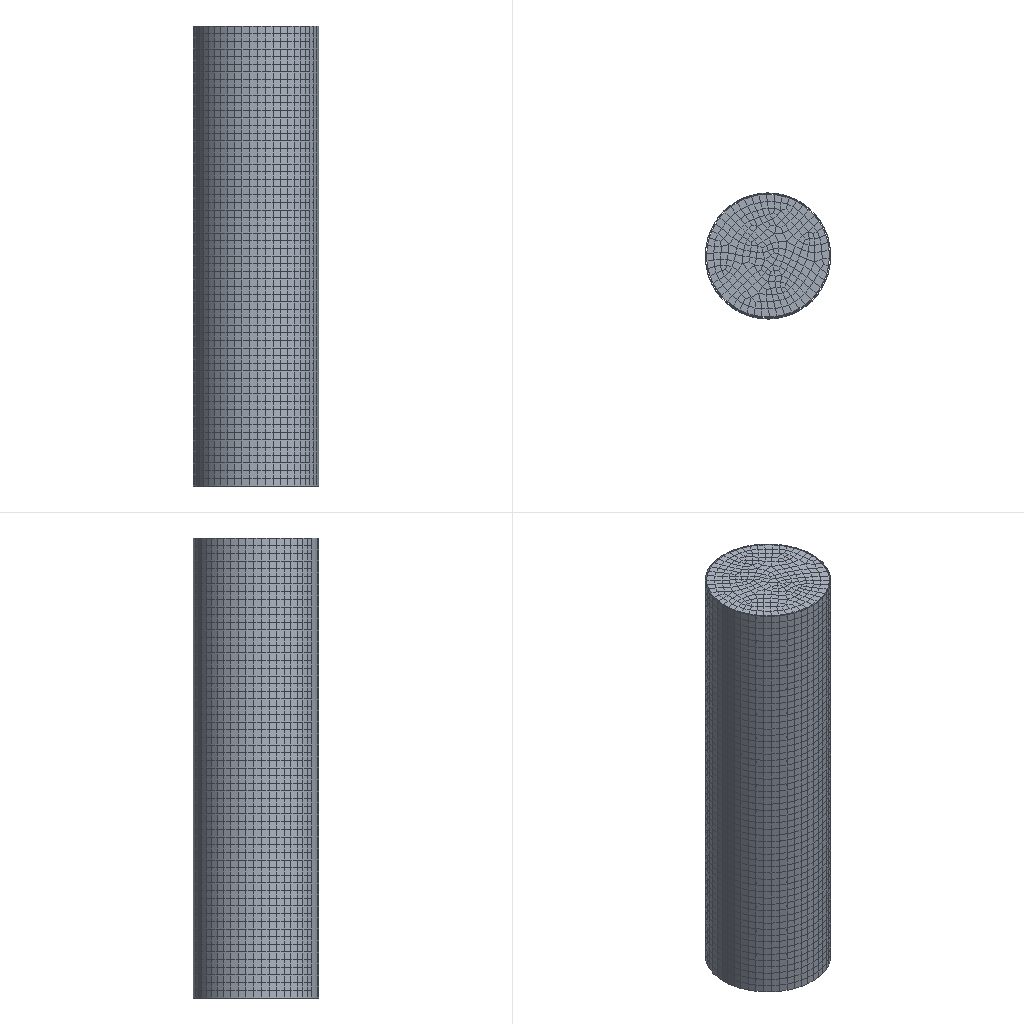Simulation study | abaqus
Set-up summary:
category,name,step,type,value,unit,region
solver,abaqus
solver,version,,,Abaqus/Standard 2020
units,not stated in the deck,,not stated
analysis,deck,,coupled temperature-displacement,coupled temperature-displacement
load_step,Step-1,Step-1,coupled temperature-displacement
load_step,requested,,,1
mesh,nodes,,,21045
mesh,elements,,,19140
element_type,S4RT,,unverified,3000
element_type,C3D8RT,,solid,16140
load,load commands in deck,,count,0
bc,support commands in deck,,count,2
material,CON,,in results
material,MATERIAL-1,,in results
check,setup vs results,,match,"per instance, exact: element labels, types and connectivity; labels of the nodes the elements use; coordinates of those nodes at SINGLE_PRECISION in 1 of 2 instance(s)"
Abaqus input file, long lists of numbers shortened:
*Heading
** Job name: Job-1 Model name: Model-1
** Generated by: Abaqus/CAE 2020
*Preprint, echo=NO, model=NO, history=NO, contact=NO
**
** PARTS
**
*Part, name=steel
*Node
      1,  0.1001, -0.368,           3.
      2, 0.05275, -0.3848,           3.
** (3048 more lines like these left out)
*Element, type=S4RT
   1,   50,    1,   51,  100
   2,    1,    2,   52,   51
** (2998 more lines like these left out)
*Nset, nset=Set-1, generate
    1,  3050,     1
*Elset, elset=Set-1, generate
    1,  3000,     1
** Section: Section-steel
*Shell Section, elset=Set-1, material=Material-1
0.018, 5
*End Part
**
*Part, name=yuanzhu
*Node
      1,  0.3146, -0.2471,           0.
      2,  0.3834, -0.1139,           0.
** (17993 more lines like these left out)
*Element, type=C3D8RT
    1,   383,   345,   344,   382,    88,    50,    49,    87
    2,   380,   342,   311,   545,    85,    47,    16,   250
** (16138 more lines like these left out)
*Nset, nset=Set-1, generate
     1,  17995,      1
*Elset, elset=Set-1, generate
     1,  16140,      1
** Section: Section-con
*Solid Section, elset=Set-1, material=con
,
*End Part
**
**
** ASSEMBLY
**
*Assembly, name=Assembly
**
*Instance, name=steel-1, part=steel
    0.05654,           0.,           0.
*End Instance
**
*Instance, name=yuanzhu-1, part=yuanzhu
*End Instance
**
*Nset, nset=Set-1, instance=yuanzhu-1, generate
     1,  17995,      1
*Elset, elset=Set-1, instance=yuanzhu-1, generate
     1,  16140,      1
*Nset, nset=Set-2, instance=steel-1, generate
    1,  3050,     1
*Elset, elset=Set-2, instance=steel-1, generate
    1,  3000,     1
*Nset, nset=Set-3, instance=steel-1, generate
    1,  3050,     1
*Nset, nset=Set-3, instance=yuanzhu-1, generate
     1,  17995,      1
*Elset, elset=Set-3, instance=steel-1, generate
    1,  3000,     1
*Elset, elset=Set-3, instance=yuanzhu-1, generate
     1,  16140,      1
*Nset, nset=Set-4, instance=steel-1, generate
 3001,  3050,     1
*Nset, nset=Set-4, instance=yuanzhu-1, generate
   1,  295,    1
*Elset, elset=Set-4, instance=steel-1, generate
 2951,  3000,     1
*Elset, elset=Set-4, instance=yuanzhu-1, generate
   1,  269,    1
*Nset, nset=Set-5, instance=steel-1, generate
    1,  3050,     1
*Nset, nset=Set-5, instance=yuanzhu-1, generate
     1,  17995,      1
*Elset, elset=Set-5, instance=steel-1, generate
    1,  3000,     1
*Elset, elset=Set-5, instance=yuanzhu-1, generate
     1,  16140,      1
*Elset, elset=_m_Surf-1_S4, internal, instance=yuanzhu-1
     1,     2,     3,     6,     7,     8,     9,    10,    12,    13,    14,    15,    16,    20,    25,    27
    33,    37,    40,    41,    42,    43,    44,    45,    48,    49,    50,    51,    56,    58,    80,   107
** (122 more lines like these left out)
*Elset, elset=_m_Surf-1_S6, internal, instance=yuanzhu-1
     4,     5,    17,    28,    31,    32,    35,    36,    39,    46,    52,    54,    61,    71,    77,    83
   273,   274,   286,   297,   300,   301,   304,   305,   308,   315,   321,   323,   330,   340,   346,   352
** (58 more lines like these left out)
*Elset, elset=_m_Surf-1_S3, internal, instance=yuanzhu-1, generate
    47,  15918,    269
*Surface, type=ELEMENT, name=m_Surf-1
_m_Surf-1_S4, S4
_m_Surf-1_S6, S6
_m_Surf-1_S3, S3
*Elset, elset=_s_Surf-1_SNEG, internal, instance=steel-1, generate
    1,  3000,     1
*Surface, type=ELEMENT, name=s_Surf-1
_s_Surf-1_SNEG, SNEG
*Elset, elset=__Int-2_gcs0_1_SPOS, internal, instance=steel-1, generate
    1,  3000,     1
*Surface, type=ELEMENT, name=_Int-2_gcs0_1, internal
__Int-2_gcs0_1_SPOS, SPOS
*Elset, elset=__Int-2_gcs0_2_SNEG, internal, instance=steel-1, generate
    1,  3000,     1
*Surface, type=ELEMENT, name=_Int-2_gcs0_2, internal
__Int-2_gcs0_2_SNEG, SNEG
*Elset, elset=__Int-2_gcs0_3_S4, internal, instance=yuanzhu-1
     1,     2,     3,     6,     7,     8,     9,    10,    12,    13,    14,    15,    16,    20,    25,    27
    33,    37,    40,    41,    42,    43,    44,    45,    48,    49,    50,    51,    56,    58,    80,   107
** (122 more lines like these left out)
*Elset, elset=__Int-2_gcs0_3_S6, internal, instance=yuanzhu-1
     4,     5,    17,    28,    31,    32,    35,    36,    39,    46,    52,    54,    61,    71,    77,    83
   273,   274,   286,   297,   300,   301,   304,   305,   308,   315,   321,   323,   330,   340,   346,   352
** (58 more lines like these left out)
*Elset, elset=__Int-2_gcs0_3_S3, internal, instance=yuanzhu-1, generate
    47,  15918,    269
*Surface, type=ELEMENT, name=_Int-2_gcs0_3, internal
__Int-2_gcs0_3_S4, S4
__Int-2_gcs0_3_S6, S6
__Int-2_gcs0_3_S3, S3
*End Assembly
**
** MATERIALS
**
*Material, name=Material-1
*Conductivity
45.,
*Density
7800.,
*Elastic
 2.06e+11, 0.3
*Expansion
 1.2e-05,
*Specific Heat
670.,
*Material, name=con
*Conductivity
 1.5,
*Density
2500.,
*Elastic
 3.45e+10, 0.2
*Expansion
 1e-05,
*Specific Heat
970.,
**
** INTERACTION PROPERTIES
**
*Surface Interaction, name=IntProp-1
1.,
*Friction, slip tolerance=0.005
 0.3,
*Surface Behavior, pressure-overclosure=HARD
**
** PREDEFINED FIELDS
**
** Name: Predefined Field-1   Type: Temperature
*Initial Conditions, type=TEMPERATURE
Set-1, 0., 0., 0., 0., 0.
** Name: Predefined Field-2   Type: Temperature
*Initial Conditions, type=TEMPERATURE
Set-5, 40., 40., 40., 40., 40.
**
** INTERACTIONS
**
** Interaction: Int-2
*Contact
*Contact Inclusions, ALL EXTERIOR
*Contact Property Assignment
 ,  , IntProp-1
*Surface Property Assignment, property=GEOMETRIC CORRECTION
_Int-2_gcs0_1, Circumferential, 3.04467e-08, 0., 0.,  3.04467e-08, 0., 1.
_Int-2_gcs0_2, Circumferential, 3.04467e-08, 0., 0.,  3.04467e-08, 0., 1.
_Int-2_gcs0_3, Circumferential, 0., 0., 0.,  0., 0., 1.
** ----------------------------------------------------------------
**
** STEP: Step-1
**
*Step, name=Step-1, nlgeom=YES, inc=1000
*Coupled Temperature-displacement, creep=none, deltmx=1e+08, stabilize=0.0002, allsdtol=0.05, continue=NO
0.01, 10., 0.0001, 1.
**
** BOUNDARY CONDITIONS
**
** Name: BC-1 Type: 温度
*Boundary
Set-3, 11, 11
** Name: BC-2 Type: 位移/转角
*Boundary
Set-4, 3, 3
**
** OUTPUT REQUESTS
**
*Restart, write, frequency=0
**
** FIELD OUTPUT: F-Output-1
**
*Output, field
*Node Output
CF, NT, RF, RFL, RM, RT, TF, U
V
*Element Output, directions=YES
E, HFL, LE, MISES, MISESMAX, NE, PE, PEEQ, PEMAG, S, SF, TEMP
*Contact Output
CDISP, CSTRESS
*Radiation Output
FTEMP,
**
** HISTORY OUTPUT: H-Output-1
**
*Output, history, variable=PRESELECT
*End Step
Results summary:
result,step,,completed,increments=20 time=10.0/10.0
result,analysis,,,"coupled temperature-displacement, steady state"
result,last_loadstep,,,1
result,primary field,,,"U, NT11"
result,reaction total,,FX,0.0,model units
result,reaction total,,FY,0.0,model units
result,reaction total,,FZ,-1.073,model units